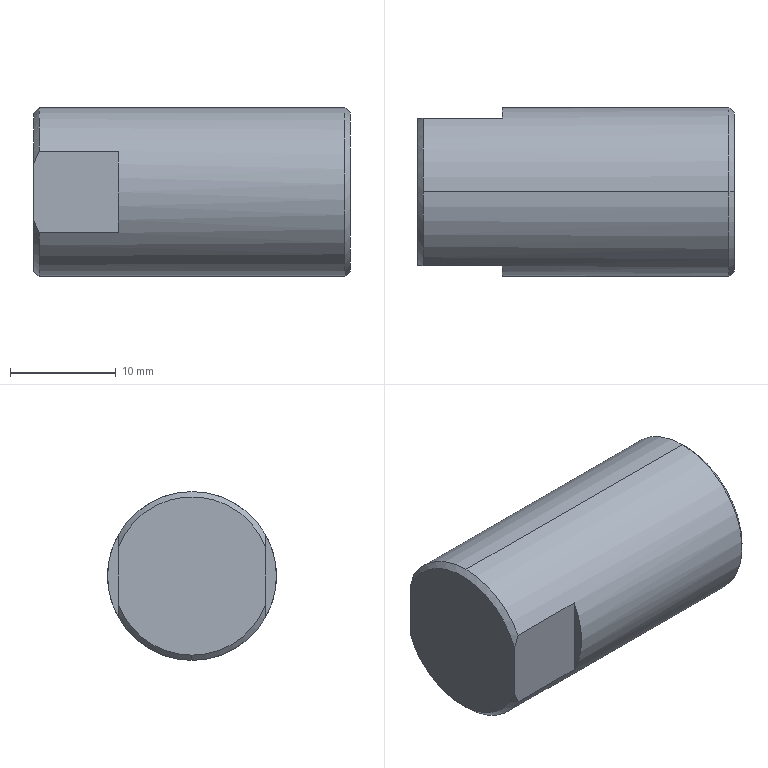Part | STEP file | PN_0024 Shaft_Default | 1 solid | 17 faces | box 30 x 16 x 16 mm | volume 5731 mm3 | cone 7 | plane 6 | cylinder 4 | commonest cylinder face diameters 5 x2 16 x2
STEP:
#1=CARTESIAN_POINT('',(0.,0.,0.));
#2=DIRECTION('',(0.,0.,1.));
#3=DIRECTION('',(1.,0.,0.));
#4=AXIS2_PLACEMENT_3D('',#1,#2,#3);
#5=CARTESIAN_POINT('',(20.,0.,-2.5));
#6=VERTEX_POINT('',#5);
#7=CARTESIAN_POINT('',(30.,0.,-2.5));
#8=VERTEX_POINT('',#7);
#9=CARTESIAN_POINT('',(30.,0.,-2.5));
#10=DIRECTION('',(1.,0.,0.));
#11=VECTOR('',#10,1.);
#12=LINE('',#9,#11);
#13=CARTESIAN_POINT('',(30.,0.,0.));
#14=DIRECTION('',(1.,0.,0.));
#15=DIRECTION('',(0.,0.,-1.));
#16=AXIS2_PLACEMENT_3D('',#13,#14,#15);
#17=CYLINDRICAL_SURFACE('',#16,2.5);
#18=CARTESIAN_POINT('',(6.283,0.));
#19=DIRECTION('',(0.,1.));
#20=VECTOR('',#19,1.);
#21=LINE('',#18,#20);
#22=(GEOMETRIC_REPRESENTATION_CONTEXT(2)PARAMETRIC_REPRESENTATION_CONTEXT()REPRESENTATION_CONTEXT('',''));
#23=DEFINITIONAL_REPRESENTATION('',(#21),#22);
#24=PCURVE('',#17,#23);
#25=CARTESIAN_POINT('',(30.,0.,0.));
#26=DIRECTION('',(1.,0.,0.));
#27=DIRECTION('',(0.,0.,-1.));
#28=AXIS2_PLACEMENT_3D('',#25,#26,#27);
#29=CYLINDRICAL_SURFACE('',#28,2.5);
#30=CARTESIAN_POINT('',(0.,0.));
#31=DIRECTION('',(0.,1.));
#32=VECTOR('',#31,1.);
#33=LINE('',#30,#32);
#34=(GEOMETRIC_REPRESENTATION_CONTEXT(2)PARAMETRIC_REPRESENTATION_CONTEXT()REPRESENTATION_CONTEXT('',''));
#35=DEFINITIONAL_REPRESENTATION('',(#33),#34);
#36=PCURVE('',#29,#35);
#37=SURFACE_CURVE('',#12,(#24,#36),.PCURVE_S1.);
#38=EDGE_CURVE('',#6,#8,#37,.T.);
#39=ORIENTED_EDGE('',*,*,#38,.T.);
#40=CARTESIAN_POINT('',(30.,0.,2.5));
#41=VERTEX_POINT('',#40);
#42=CARTESIAN_POINT('',(30.,0.,0.));
#43=DIRECTION('',(1.,0.,0.));
#44=DIRECTION('',(0.,0.,-1.));
#45=AXIS2_PLACEMENT_3D('',#42,#43,#44);
#46=CIRCLE('',#45,2.5);
#47=CARTESIAN_POINT('',(0.,0.));
#48=DIRECTION('',(1.,0.));
#49=VECTOR('',#48,1.);
#50=LINE('',#47,#49);
#51=(GEOMETRIC_REPRESENTATION_CONTEXT(2)PARAMETRIC_REPRESENTATION_CONTEXT()REPRESENTATION_CONTEXT('',''));
#52=DEFINITIONAL_REPRESENTATION('',(#50),#51);
#53=PCURVE('',#17,#52);
#54=CARTESIAN_POINT('',(30.,0.,0.));
#55=DIRECTION('',(1.,0.,0.));
#56=DIRECTION('',(0.,0.,-1.));
#57=AXIS2_PLACEMENT_3D('',#54,#55,#56);
#58=PLANE('',#57);
#59=CARTESIAN_POINT('',(0.,0.));
#60=DIRECTION('',(1.,0.));
#61=AXIS2_PLACEMENT_2D('',#59,#60);
#62=CIRCLE('',#61,2.5);
#63=(GEOMETRIC_REPRESENTATION_CONTEXT(2)PARAMETRIC_REPRESENTATION_CONTEXT()REPRESENTATION_CONTEXT('',''));
#64=DEFINITIONAL_REPRESENTATION('',(#62),#63);
#65=PCURVE('',#58,#64);
#66=SURFACE_CURVE('',#46,(#53,#65),.PCURVE_S1.);
#67=EDGE_CURVE('',#41,#8,#66,.T.);
#68=ORIENTED_EDGE('',*,*,#67,.F.);
#69=CARTESIAN_POINT('',(20.,0.,2.5));
#70=VERTEX_POINT('',#69);
#71=CARTESIAN_POINT('',(30.,0.,2.5));
#72=DIRECTION('',(1.,0.,0.));
#73=VECTOR('',#72,1.);
#74=LINE('',#71,#73);
#75=CARTESIAN_POINT('',(3.142,0.));
#76=DIRECTION('',(0.,1.));
#77=VECTOR('',#76,1.);
#78=LINE('',#75,#77);
#79=(GEOMETRIC_REPRESENTATION_CONTEXT(2)PARAMETRIC_REPRESENTATION_CONTEXT()REPRESENTATION_CONTEXT('',''));
#80=DEFINITIONAL_REPRESENTATION('',(#78),#79);
#81=PCURVE('',#17,#80);
#82=CARTESIAN_POINT('',(3.142,0.));
#83=DIRECTION('',(0.,1.));
#84=VECTOR('',#83,1.);
#85=LINE('',#82,#84);
#86=(GEOMETRIC_REPRESENTATION_CONTEXT(2)PARAMETRIC_REPRESENTATION_CONTEXT()REPRESENTATION_CONTEXT('',''));
#87=DEFINITIONAL_REPRESENTATION('',(#85),#86);
#88=PCURVE('',#29,#87);
#89=SURFACE_CURVE('',#74,(#81,#88),.PCURVE_S1.);
#90=EDGE_CURVE('',#70,#41,#89,.T.);
#91=ORIENTED_EDGE('',*,*,#90,.F.);
#92=CARTESIAN_POINT('',(20.,0.,0.));
#93=DIRECTION('',(1.,0.,0.));
#94=DIRECTION('',(0.,0.,-1.));
#95=AXIS2_PLACEMENT_3D('',#92,#93,#94);
#96=CIRCLE('',#95,2.5);
#97=CARTESIAN_POINT('',(0.,-10.));
#98=DIRECTION('',(1.,0.));
#99=VECTOR('',#98,1.);
#100=LINE('',#97,#99);
#101=(GEOMETRIC_REPRESENTATION_CONTEXT(2)PARAMETRIC_REPRESENTATION_CONTEXT()REPRESENTATION_CONTEXT('',''));
#102=DEFINITIONAL_REPRESENTATION('',(#100),#101);
#103=PCURVE('',#17,#102);
#104=CARTESIAN_POINT('',(20.,0.,0.));
#105=DIRECTION('',(1.,0.,0.));
#106=DIRECTION('',(0.,0.,-1.));
#107=AXIS2_PLACEMENT_3D('',#104,#105,#106);
#108=CONICAL_SURFACE('',#107,2.5,1.03);
#109=CARTESIAN_POINT('',(0.,0.));
#110=DIRECTION('',(1.,0.));
#111=VECTOR('',#110,1.);
#112=LINE('',#109,#111);
#113=(GEOMETRIC_REPRESENTATION_CONTEXT(2)PARAMETRIC_REPRESENTATION_CONTEXT()REPRESENTATION_CONTEXT('',''));
#114=DEFINITIONAL_REPRESENTATION('',(#112),#113);
#115=PCURVE('',#108,#114);
#116=SURFACE_CURVE('',#96,(#103,#115),.PCURVE_S1.);
#117=EDGE_CURVE('',#70,#6,#116,.T.);
#118=ORIENTED_EDGE('',*,*,#117,.T.);
#119=EDGE_LOOP('',(#39,#68,#91,#118));
#120=FACE_BOUND('',#119,.F.);
#121=ADVANCED_FACE('',(#120),#17,.F.);
#122=ORIENTED_EDGE('',*,*,#117,.F.);
#123=CARTESIAN_POINT('',(18.498,0.,0.));
#124=VERTEX_POINT('',#123);
#125=CARTESIAN_POINT('',(20.,0.,2.5));
#126=DIRECTION('',(0.515,0.,0.8572));
#127=VECTOR('',#126,1.);
#128=LINE('',#125,#127);
#129=CARTESIAN_POINT('',(3.142,0.));
#130=DIRECTION('',(0.,1.));
#131=VECTOR('',#130,1.);
#132=LINE('',#129,#131);
#133=(GEOMETRIC_REPRESENTATION_CONTEXT(2)PARAMETRIC_REPRESENTATION_CONTEXT()REPRESENTATION_CONTEXT('',''));
#134=DEFINITIONAL_REPRESENTATION('',(#132),#133);
#135=PCURVE('',#108,#134);
#136=CARTESIAN_POINT('',(20.,0.,0.));
#137=DIRECTION('',(1.,0.,0.));
#138=DIRECTION('',(0.,0.,-1.));
#139=AXIS2_PLACEMENT_3D('',#136,#137,#138);
#140=CONICAL_SURFACE('',#139,2.5,1.03);
#141=CARTESIAN_POINT('',(3.142,0.));
#142=DIRECTION('',(0.,1.));
#143=VECTOR('',#142,1.);
#144=LINE('',#141,#143);
#145=(GEOMETRIC_REPRESENTATION_CONTEXT(2)PARAMETRIC_REPRESENTATION_CONTEXT()REPRESENTATION_CONTEXT('',''));
#146=DEFINITIONAL_REPRESENTATION('',(#144),#145);
#147=PCURVE('',#140,#146);
#148=SURFACE_CURVE('',#128,(#135,#147),.PCURVE_S1.);
#149=EDGE_CURVE('',#124,#70,#148,.T.);
#150=ORIENTED_EDGE('',*,*,#149,.F.);
#151=CARTESIAN_POINT('',(20.,0.,-2.5));
#152=DIRECTION('',(0.515,0.,-0.8572));
#153=VECTOR('',#152,1.);
#154=LINE('',#151,#153);
#155=CARTESIAN_POINT('',(6.283,-1.502));
#156=CARTESIAN_POINT('',(6.283,-1.479));
#157=CARTESIAN_POINT('',(6.283,-1.434));
#158=CARTESIAN_POINT('',(6.283,-1.366));
#159=CARTESIAN_POINT('',(6.283,-1.297));
#160=CARTESIAN_POINT('',(6.283,-1.229));
#161=CARTESIAN_POINT('',(6.283,-1.161));
#162=CARTESIAN_POINT('',(6.283,-1.092));
#163=CARTESIAN_POINT('',(6.283,-1.024));
#164=CARTESIAN_POINT('',(6.283,-0.9559));
#165=CARTESIAN_POINT('',(6.283,-0.8876));
#166=CARTESIAN_POINT('',(6.283,-0.8194));
#167=CARTESIAN_POINT('',(6.283,-0.7511));
#168=CARTESIAN_POINT('',(6.283,-0.6828));
#169=CARTESIAN_POINT('',(6.283,-0.6145));
#170=CARTESIAN_POINT('',(6.283,-0.5462));
#171=CARTESIAN_POINT('',(6.283,-0.478));
#172=CARTESIAN_POINT('',(6.283,-0.4097));
#173=CARTESIAN_POINT('',(6.283,-0.3414));
#174=CARTESIAN_POINT('',(6.283,-0.2731));
#175=CARTESIAN_POINT('',(6.283,-0.2048));
#176=CARTESIAN_POINT('',(6.283,-0.1366));
#177=CARTESIAN_POINT('',(6.283,-0.06828));
#178=CARTESIAN_POINT('',(6.283,-0.02276));
#179=CARTESIAN_POINT('',(6.283,0.));
#180=B_SPLINE_CURVE_WITH_KNOTS('',3,(#155,#156,#157,#158,#159,#160,#161,#162,#163,#164,#165,#166,#167,#168,#169,#170,#171,#172,#173,#174,#175,#176,#177,#178,#179),.UNSPECIFIED.,.F.,.F.,(4,1,1,1,1,1,1,1,1,1,1,1,1,1,1,1,1,1,1,1,1,1,4),(-2.917,-2.784,-2.651,-2.519,-2.386,-2.254,-2.121,-1.989,-1.856,-1.723,-1.591,-1.458,-1.326,-1.193,-1.061,-0.928,-0.7954,-0.6629,-0.5303,-0.3977,-0.2651,-0.1326,0.),.UNSPECIFIED.);
#181=(GEOMETRIC_REPRESENTATION_CONTEXT(2)PARAMETRIC_REPRESENTATION_CONTEXT()REPRESENTATION_CONTEXT('',''));
#182=DEFINITIONAL_REPRESENTATION('',(#180),#181);
#183=PCURVE('',#108,#182);
#184=CARTESIAN_POINT('',(0.,0.));
#185=DIRECTION('',(0.,1.));
#186=VECTOR('',#185,1.);
#187=LINE('',#184,#186);
#188=(GEOMETRIC_REPRESENTATION_CONTEXT(2)PARAMETRIC_REPRESENTATION_CONTEXT()REPRESENTATION_CONTEXT('',''));
#189=DEFINITIONAL_REPRESENTATION('',(#187),#188);
#190=PCURVE('',#140,#189);
#191=SURFACE_CURVE('',#154,(#183,#190),.PCURVE_S1.);
#192=EDGE_CURVE('',#124,#6,#191,.T.);
#193=ORIENTED_EDGE('',*,*,#192,.T.);
#194=EDGE_LOOP('',(#122,#150,#193));
#195=FACE_BOUND('',#194,.F.);
#196=ADVANCED_FACE('',(#195),#108,.F.);
#197=CARTESIAN_POINT('',(0.,0.,-7.5));
#198=VERTEX_POINT('',#197);
#199=CARTESIAN_POINT('',(0.,-7.,-2.693));
#200=VERTEX_POINT('',#199);
#201=CARTESIAN_POINT('',(0.,0.,0.));
#202=DIRECTION('',(-1.,0.,0.));
#203=DIRECTION('',(0.,0.,-1.));
#204=AXIS2_PLACEMENT_3D('',#201,#202,#203);
#205=CIRCLE('',#204,7.5);
#206=CARTESIAN_POINT('',(0.5,0.,0.));
#207=DIRECTION('',(1.,0.,0.));
#208=DIRECTION('',(0.,0.,-1.));
#209=AXIS2_PLACEMENT_3D('',#206,#207,#208);
#210=CONICAL_SURFACE('',#209,8.,0.7854);
#211=CARTESIAN_POINT('',(6.283,-0.5));
#212=DIRECTION('',(-1.,0.));
#213=VECTOR('',#212,1.);
#214=LINE('',#211,#213);
#215=(GEOMETRIC_REPRESENTATION_CONTEXT(2)PARAMETRIC_REPRESENTATION_CONTEXT()REPRESENTATION_CONTEXT('',''));
#216=DEFINITIONAL_REPRESENTATION('',(#214),#215);
#217=PCURVE('',#210,#216);
#218=CARTESIAN_POINT('',(0.,0.,0.));
#219=DIRECTION('',(1.,0.,0.));
#220=DIRECTION('',(0.,0.,-1.));
#221=AXIS2_PLACEMENT_3D('',#218,#219,#220);
#222=PLANE('',#221);
#223=CARTESIAN_POINT('',(7.5,0.));
#224=CARTESIAN_POINT('',(7.5,-12.99));
#225=CARTESIAN_POINT('',(-3.75,-6.495));
#226=CARTESIAN_POINT('',(-15.,0.));
#227=CARTESIAN_POINT('',(-3.75,6.495));
#228=CARTESIAN_POINT('',(7.5,12.99));
#229=CARTESIAN_POINT('',(7.5,0.));
#230=(BOUNDED_CURVE()B_SPLINE_CURVE(2,(#223,#224,#225,#226,#227,#228,#229),.UNSPECIFIED.,.T.,.F.)B_SPLINE_CURVE_WITH_KNOTS((1,2,2,2,2,1),(-2.094,0.,2.094,4.189,6.283,8.378),.UNSPECIFIED.)CURVE()GEOMETRIC_REPRESENTATION_ITEM()RATIONAL_B_SPLINE_CURVE((1.,0.5,1.,0.5,1.,0.5,1.))REPRESENTATION_ITEM(''));
#231=(GEOMETRIC_REPRESENTATION_CONTEXT(2)PARAMETRIC_REPRESENTATION_CONTEXT()REPRESENTATION_CONTEXT('',''));
#232=DEFINITIONAL_REPRESENTATION('',(#230),#231);
#233=PCURVE('',#222,#232);
#234=SURFACE_CURVE('',#205,(#217,#233),.PCURVE_S1.);
#235=EDGE_CURVE('',#198,#200,#234,.T.);
#236=ORIENTED_EDGE('',*,*,#235,.F.);
#237=CARTESIAN_POINT('',(0.5,0.,-8.));
#238=VERTEX_POINT('',#237);
#239=CARTESIAN_POINT('',(0.5,0.,-8.));
#240=DIRECTION('',(0.7071,0.,-0.7071));
#241=VECTOR('',#240,1.);
#242=LINE('',#239,#241);
#243=CARTESIAN_POINT('',(6.283,0.));
#244=DIRECTION('',(0.,1.));
#245=VECTOR('',#244,1.);
#246=LINE('',#243,#245);
#247=(GEOMETRIC_REPRESENTATION_CONTEXT(2)PARAMETRIC_REPRESENTATION_CONTEXT()REPRESENTATION_CONTEXT('',''));
#248=DEFINITIONAL_REPRESENTATION('',(#246),#247);
#249=PCURVE('',#210,#248);
#250=CARTESIAN_POINT('',(0.5,0.,0.));
#251=DIRECTION('',(1.,0.,0.));
#252=DIRECTION('',(0.,0.,-1.));
#253=AXIS2_PLACEMENT_3D('',#250,#251,#252);
#254=CONICAL_SURFACE('',#253,8.,0.7854);
#255=CARTESIAN_POINT('',(0.,0.));
#256=DIRECTION('',(0.,1.));
#257=VECTOR('',#256,1.);
#258=LINE('',#255,#257);
#259=(GEOMETRIC_REPRESENTATION_CONTEXT(2)PARAMETRIC_REPRESENTATION_CONTEXT()REPRESENTATION_CONTEXT('',''));
#260=DEFINITIONAL_REPRESENTATION('',(#258),#259);
#261=PCURVE('',#254,#260);
#262=SURFACE_CURVE('',#242,(#249,#261),.PCURVE_S1.);
#263=EDGE_CURVE('',#198,#238,#262,.T.);
#264=ORIENTED_EDGE('',*,*,#263,.T.);
#265=CARTESIAN_POINT('',(0.5,-7.,-3.873));
#266=VERTEX_POINT('',#265);
#267=CARTESIAN_POINT('',(0.5,0.,0.));
#268=DIRECTION('',(1.,0.,0.));
#269=DIRECTION('',(0.,0.,-1.));
#270=AXIS2_PLACEMENT_3D('',#267,#268,#269);
#271=CIRCLE('',#270,8.);
#272=CARTESIAN_POINT('',(0.,0.));
#273=DIRECTION('',(1.,0.));
#274=VECTOR('',#273,1.);
#275=LINE('',#272,#274);
#276=(GEOMETRIC_REPRESENTATION_CONTEXT(2)PARAMETRIC_REPRESENTATION_CONTEXT()REPRESENTATION_CONTEXT('',''));
#277=DEFINITIONAL_REPRESENTATION('',(#275),#276);
#278=PCURVE('',#210,#277);
#279=CARTESIAN_POINT('',(30.,0.,0.));
#280=DIRECTION('',(-1.,0.,0.));
#281=DIRECTION('',(0.,0.,1.));
#282=AXIS2_PLACEMENT_3D('',#279,#280,#281);
#283=CYLINDRICAL_SURFACE('',#282,8.);
#284=CARTESIAN_POINT('',(9.425,29.5));
#285=DIRECTION('',(-1.,0.));
#286=VECTOR('',#285,1.);
#287=LINE('',#284,#286);
#288=(GEOMETRIC_REPRESENTATION_CONTEXT(2)PARAMETRIC_REPRESENTATION_CONTEXT()REPRESENTATION_CONTEXT('',''));
#289=DEFINITIONAL_REPRESENTATION('',(#287),#288);
#290=PCURVE('',#283,#289);
#291=SURFACE_CURVE('',#271,(#278,#290),.PCURVE_S1.);
#292=EDGE_CURVE('',#266,#238,#291,.T.);
#293=ORIENTED_EDGE('',*,*,#292,.F.);
#294=CARTESIAN_POINT('',(0.,-7.,-2.693));
#295=CARTESIAN_POINT('',(0.1454,-7.,-3.098));
#296=CARTESIAN_POINT('',(0.3148,-7.,-3.491));
#297=CARTESIAN_POINT('',(0.5,-7.,-3.873));
#298=B_SPLINE_CURVE_WITH_KNOTS('',3,(#294,#295,#296,#297),.UNSPECIFIED.,.F.,.F.,(4,4),(0.02242,0.02371),.PIECEWISE_BEZIER_KNOTS.);
#299=CARTESIAN_POINT('',(5.08,-0.5));
#300=CARTESIAN_POINT('',(5.082,-0.4934));
#301=CARTESIAN_POINT('',(5.086,-0.4801));
#302=CARTESIAN_POINT('',(5.093,-0.4598));
#303=CARTESIAN_POINT('',(5.1,-0.4392));
#304=CARTESIAN_POINT('',(5.107,-0.4184));
#305=CARTESIAN_POINT('',(5.113,-0.3973));
#306=CARTESIAN_POINT('',(5.12,-0.3759));
#307=CARTESIAN_POINT('',(5.126,-0.3542));
#308=CARTESIAN_POINT('',(5.133,-0.3323));
#309=CARTESIAN_POINT('',(5.139,-0.3101));
#310=CARTESIAN_POINT('',(5.146,-0.2876));
#311=CARTESIAN_POINT('',(5.152,-0.2649));
#312=CARTESIAN_POINT('',(5.158,-0.242));
#313=CARTESIAN_POINT('',(5.164,-0.2188));
#314=CARTESIAN_POINT('',(5.17,-0.1954));
#315=CARTESIAN_POINT('',(5.177,-0.1717));
#316=CARTESIAN_POINT('',(5.183,-0.1478));
#317=CARTESIAN_POINT('',(5.189,-0.1237));
#318=CARTESIAN_POINT('',(5.195,-0.09942));
#319=CARTESIAN_POINT('',(5.2,-0.07488));
#320=CARTESIAN_POINT('',(5.206,-0.05013));
#321=CARTESIAN_POINT('',(5.212,-0.02518));
#322=CARTESIAN_POINT('',(5.216,-0.008416));
#323=CARTESIAN_POINT('',(5.218,0.));
#324=B_SPLINE_CURVE_WITH_KNOTS('',3,(#299,#300,#301,#302,#303,#304,#305,#306,#307,#308,#309,#310,#311,#312,#313,#314,#315,#316,#317,#318,#319,#320,#321,#322,#323),.UNSPECIFIED.,.F.,.F.,(4,1,1,1,1,1,1,1,1,1,1,1,1,1,1,1,1,1,1,1,1,1,4),(0.02242,0.02248,0.02254,0.0226,0.02266,0.02272,0.02277,0.02283,0.02289,0.02295,0.02301,0.02307,0.02312,0.02318,0.02324,0.0233,0.02336,0.02342,0.02347,0.02353,0.02359,0.02365,0.02371),.QUASI_UNIFORM_KNOTS.);
#325=(GEOMETRIC_REPRESENTATION_CONTEXT(2)PARAMETRIC_REPRESENTATION_CONTEXT()REPRESENTATION_CONTEXT('',''));
#326=DEFINITIONAL_REPRESENTATION('',(#324),#325);
#327=PCURVE('',#210,#326);
#328=CARTESIAN_POINT('',(0.,-7.,-18.));
#329=DIRECTION('',(0.,1.,0.));
#330=DIRECTION('',(0.,0.,1.));
#331=AXIS2_PLACEMENT_3D('',#328,#329,#330);
#332=PLANE('',#331);
#333=CARTESIAN_POINT('',(15.307,0.));
#334=CARTESIAN_POINT('',(14.902,0.1454));
#335=CARTESIAN_POINT('',(14.509,0.3148));
#336=CARTESIAN_POINT('',(14.127,0.5));
#337=B_SPLINE_CURVE_WITH_KNOTS('',3,(#333,#334,#335,#336),.UNSPECIFIED.,.F.,.F.,(4,4),(0.02242,0.02371),.PIECEWISE_BEZIER_KNOTS.);
#338=(GEOMETRIC_REPRESENTATION_CONTEXT(2)PARAMETRIC_REPRESENTATION_CONTEXT()REPRESENTATION_CONTEXT('',''));
#339=DEFINITIONAL_REPRESENTATION('',(#337),#338);
#340=PCURVE('',#332,#339);
#341=SURFACE_CURVE('',#298,(#327,#340),.PCURVE_S1.);
#342=EDGE_CURVE('',#200,#266,#341,.T.);
#343=ORIENTED_EDGE('',*,*,#342,.F.);
#344=EDGE_LOOP('',(#236,#264,#293,#343));
#345=FACE_BOUND('',#344,.T.);
#346=ADVANCED_FACE('',(#345),#210,.T.);
#347=CARTESIAN_POINT('',(30.,0.,-7.5));
#348=VERTEX_POINT('',#347);
#349=CARTESIAN_POINT('',(30.,0.,7.5));
#350=VERTEX_POINT('',#349);
#351=CARTESIAN_POINT('',(30.,0.,0.));
#352=DIRECTION('',(1.,0.,0.));
#353=DIRECTION('',(0.,0.,-1.));
#354=AXIS2_PLACEMENT_3D('',#351,#352,#353);
#355=CIRCLE('',#354,7.5);
#356=CARTESIAN_POINT('',(30.,0.,0.));
#357=DIRECTION('',(-1.,0.,0.));
#358=DIRECTION('',(0.,0.,1.));
#359=AXIS2_PLACEMENT_3D('',#356,#357,#358);
#360=CONICAL_SURFACE('',#359,7.5,0.7854);
#361=CARTESIAN_POINT('',(3.142,0.));
#362=DIRECTION('',(-1.,0.));
#363=VECTOR('',#362,1.);
#364=LINE('',#361,#363);
#365=(GEOMETRIC_REPRESENTATION_CONTEXT(2)PARAMETRIC_REPRESENTATION_CONTEXT()REPRESENTATION_CONTEXT('',''));
#366=DEFINITIONAL_REPRESENTATION('',(#364),#365);
#367=PCURVE('',#360,#366);
#368=CARTESIAN_POINT('',(0.,0.));
#369=DIRECTION('',(1.,0.));
#370=AXIS2_PLACEMENT_2D('',#368,#369);
#371=CIRCLE('',#370,7.5);
#372=(GEOMETRIC_REPRESENTATION_CONTEXT(2)PARAMETRIC_REPRESENTATION_CONTEXT()REPRESENTATION_CONTEXT('',''));
#373=DEFINITIONAL_REPRESENTATION('',(#371),#372);
#374=PCURVE('',#58,#373);
#375=SURFACE_CURVE('',#355,(#367,#374),.PCURVE_S1.);
#376=EDGE_CURVE('',#348,#350,#375,.T.);
#377=ORIENTED_EDGE('',*,*,#376,.F.);
#378=CARTESIAN_POINT('',(29.5,0.,-8.));
#379=VERTEX_POINT('',#378);
#380=CARTESIAN_POINT('',(30.,0.,-7.5));
#381=DIRECTION('',(-0.7071,0.,-0.7071));
#382=VECTOR('',#381,1.);
#383=LINE('',#380,#382);
#384=CARTESIAN_POINT('',(3.142,0.));
#385=DIRECTION('',(0.,1.));
#386=VECTOR('',#385,1.);
#387=LINE('',#384,#386);
#388=(GEOMETRIC_REPRESENTATION_CONTEXT(2)PARAMETRIC_REPRESENTATION_CONTEXT()REPRESENTATION_CONTEXT('',''));
#389=DEFINITIONAL_REPRESENTATION('',(#387),#388);
#390=PCURVE('',#360,#389);
#391=CARTESIAN_POINT('',(30.,0.,0.));
#392=DIRECTION('',(-1.,0.,0.));
#393=DIRECTION('',(0.,0.,1.));
#394=AXIS2_PLACEMENT_3D('',#391,#392,#393);
#395=CONICAL_SURFACE('',#394,7.5,0.7854);
#396=CARTESIAN_POINT('',(3.142,0.));
#397=DIRECTION('',(0.,1.));
#398=VECTOR('',#397,1.);
#399=LINE('',#396,#398);
#400=(GEOMETRIC_REPRESENTATION_CONTEXT(2)PARAMETRIC_REPRESENTATION_CONTEXT()REPRESENTATION_CONTEXT('',''));
#401=DEFINITIONAL_REPRESENTATION('',(#399),#400);
#402=PCURVE('',#395,#401);
#403=SURFACE_CURVE('',#383,(#390,#402),.PCURVE_S1.);
#404=EDGE_CURVE('',#348,#379,#403,.T.);
#405=ORIENTED_EDGE('',*,*,#404,.T.);
#406=CARTESIAN_POINT('',(29.5,0.,8.));
#407=VERTEX_POINT('',#406);
#408=CARTESIAN_POINT('',(29.5,0.,0.));
#409=DIRECTION('',(-1.,0.,0.));
#410=DIRECTION('',(0.,0.,-1.));
#411=AXIS2_PLACEMENT_3D('',#408,#409,#410);
#412=CIRCLE('',#411,8.);
#413=CARTESIAN_POINT('',(-3.142,0.5));
#414=DIRECTION('',(1.,0.));
#415=VECTOR('',#414,1.);
#416=LINE('',#413,#415);
#417=(GEOMETRIC_REPRESENTATION_CONTEXT(2)PARAMETRIC_REPRESENTATION_CONTEXT()REPRESENTATION_CONTEXT('',''));
#418=DEFINITIONAL_REPRESENTATION('',(#416),#417);
#419=PCURVE('',#360,#418);
#420=CARTESIAN_POINT('',(30.,0.,0.));
#421=DIRECTION('',(-1.,0.,0.));
#422=DIRECTION('',(0.,0.,1.));
#423=AXIS2_PLACEMENT_3D('',#420,#421,#422);
#424=CYLINDRICAL_SURFACE('',#423,8.);
#425=CARTESIAN_POINT('',(-3.142,0.5));
#426=DIRECTION('',(1.,0.));
#427=VECTOR('',#426,1.);
#428=LINE('',#425,#427);
#429=(GEOMETRIC_REPRESENTATION_CONTEXT(2)PARAMETRIC_REPRESENTATION_CONTEXT()REPRESENTATION_CONTEXT('',''));
#430=DEFINITIONAL_REPRESENTATION('',(#428),#429);
#431=PCURVE('',#424,#430);
#432=SURFACE_CURVE('',#412,(#419,#431),.PCURVE_S1.);
#433=EDGE_CURVE('',#407,#379,#432,.T.);
#434=ORIENTED_EDGE('',*,*,#433,.F.);
#435=CARTESIAN_POINT('',(30.,0.,7.5));
#436=DIRECTION('',(-0.7071,0.,0.7071));
#437=VECTOR('',#436,1.);
#438=LINE('',#435,#437);
#439=CARTESIAN_POINT('',(0.,0.));
#440=DIRECTION('',(0.,1.));
#441=VECTOR('',#440,1.);
#442=LINE('',#439,#441);
#443=(GEOMETRIC_REPRESENTATION_CONTEXT(2)PARAMETRIC_REPRESENTATION_CONTEXT()REPRESENTATION_CONTEXT('',''));
#444=DEFINITIONAL_REPRESENTATION('',(#442),#443);
#445=PCURVE('',#360,#444);
#446=CARTESIAN_POINT('',(6.283,0.));
#447=DIRECTION('',(0.,1.));
#448=VECTOR('',#447,1.);
#449=LINE('',#446,#448);
#450=(GEOMETRIC_REPRESENTATION_CONTEXT(2)PARAMETRIC_REPRESENTATION_CONTEXT()REPRESENTATION_CONTEXT('',''));
#451=DEFINITIONAL_REPRESENTATION('',(#449),#450);
#452=PCURVE('',#395,#451);
#453=SURFACE_CURVE('',#438,(#445,#452),.PCURVE_S1.);
#454=EDGE_CURVE('',#350,#407,#453,.T.);
#455=ORIENTED_EDGE('',*,*,#454,.F.);
#456=EDGE_LOOP('',(#377,#405,#434,#455));
#457=FACE_BOUND('',#456,.T.);
#458=ADVANCED_FACE('',(#457),#360,.T.);
#459=ORIENTED_EDGE('',*,*,#433,.T.);
#460=CARTESIAN_POINT('',(30.,0.,-8.));
#461=DIRECTION('',(-1.,0.,0.));
#462=VECTOR('',#461,1.);
#463=LINE('',#460,#462);
#464=CARTESIAN_POINT('',(3.142,0.));
#465=DIRECTION('',(0.,1.));
#466=VECTOR('',#465,1.);
#467=LINE('',#464,#466);
#468=(GEOMETRIC_REPRESENTATION_CONTEXT(2)PARAMETRIC_REPRESENTATION_CONTEXT()REPRESENTATION_CONTEXT('',''));
#469=DEFINITIONAL_REPRESENTATION('',(#467),#468);
#470=PCURVE('',#424,#469);
#471=CARTESIAN_POINT('',(3.142,0.));
#472=DIRECTION('',(0.,1.));
#473=VECTOR('',#472,1.);
#474=LINE('',#471,#473);
#475=(GEOMETRIC_REPRESENTATION_CONTEXT(2)PARAMETRIC_REPRESENTATION_CONTEXT()REPRESENTATION_CONTEXT('',''));
#476=DEFINITIONAL_REPRESENTATION('',(#474),#475);
#477=PCURVE('',#283,#476);
#478=SURFACE_CURVE('',#463,(#470,#477),.PCURVE_S1.);
#479=EDGE_CURVE('',#379,#238,#478,.T.);
#480=ORIENTED_EDGE('',*,*,#479,.T.);
#481=CARTESIAN_POINT('',(0.5,7.,-3.873));
#482=VERTEX_POINT('',#481);
#483=CARTESIAN_POINT('',(0.5,0.,0.));
#484=DIRECTION('',(1.,0.,0.));
#485=DIRECTION('',(0.,0.,-1.));
#486=AXIS2_PLACEMENT_3D('',#483,#484,#485);
#487=CIRCLE('',#486,8.);
#488=CARTESIAN_POINT('',(3.142,29.5));
#489=DIRECTION('',(-1.,0.));
#490=VECTOR('',#489,1.);
#491=LINE('',#488,#490);
#492=(GEOMETRIC_REPRESENTATION_CONTEXT(2)PARAMETRIC_REPRESENTATION_CONTEXT()REPRESENTATION_CONTEXT('',''));
#493=DEFINITIONAL_REPRESENTATION('',(#491),#492);
#494=PCURVE('',#424,#493);
#495=CARTESIAN_POINT('',(0.,0.));
#496=DIRECTION('',(1.,0.));
#497=VECTOR('',#496,1.);
#498=LINE('',#495,#497);
#499=(GEOMETRIC_REPRESENTATION_CONTEXT(2)PARAMETRIC_REPRESENTATION_CONTEXT()REPRESENTATION_CONTEXT('',''));
#500=DEFINITIONAL_REPRESENTATION('',(#498),#499);
#501=PCURVE('',#254,#500);
#502=SURFACE_CURVE('',#487,(#494,#501),.PCURVE_S1.);
#503=EDGE_CURVE('',#238,#482,#502,.T.);
#504=ORIENTED_EDGE('',*,*,#503,.T.);
#505=CARTESIAN_POINT('',(8.,7.,-3.873));
#506=VERTEX_POINT('',#505);
#507=CARTESIAN_POINT('',(30.,7.,-3.873));
#508=DIRECTION('',(1.,0.,0.));
#509=VECTOR('',#508,1.);
#510=LINE('',#507,#509);
#511=CARTESIAN_POINT('',(2.076,0.));
#512=DIRECTION('',(0.,-1.));
#513=VECTOR('',#512,1.);
#514=LINE('',#511,#513);
#515=(GEOMETRIC_REPRESENTATION_CONTEXT(2)PARAMETRIC_REPRESENTATION_CONTEXT()REPRESENTATION_CONTEXT('',''));
#516=DEFINITIONAL_REPRESENTATION('',(#514),#515);
#517=PCURVE('',#424,#516);
#518=CARTESIAN_POINT('',(0.,7.,-18.));
#519=DIRECTION('',(0.,-1.,0.));
#520=DIRECTION('',(0.,0.,-1.));
#521=AXIS2_PLACEMENT_3D('',#518,#519,#520);
#522=PLANE('',#521);
#523=CARTESIAN_POINT('',(-14.127,30.));
#524=DIRECTION('',(0.,1.));
#525=VECTOR('',#524,1.);
#526=LINE('',#523,#525);
#527=(GEOMETRIC_REPRESENTATION_CONTEXT(2)PARAMETRIC_REPRESENTATION_CONTEXT()REPRESENTATION_CONTEXT('',''));
#528=DEFINITIONAL_REPRESENTATION('',(#526),#527);
#529=PCURVE('',#522,#528);
#530=SURFACE_CURVE('',#510,(#517,#529),.PCURVE_S1.);
#531=EDGE_CURVE('',#482,#506,#530,.T.);
#532=ORIENTED_EDGE('',*,*,#531,.T.);
#533=CARTESIAN_POINT('',(8.,7.,3.873));
#534=VERTEX_POINT('',#533);
#535=CARTESIAN_POINT('',(8.,0.,0.));
#536=DIRECTION('',(1.,0.,0.));
#537=DIRECTION('',(0.,0.,-1.));
#538=AXIS2_PLACEMENT_3D('',#535,#536,#537);
#539=CIRCLE('',#538,8.);
#540=CARTESIAN_POINT('',(3.142,22.));
#541=DIRECTION('',(-1.,0.));
#542=VECTOR('',#541,1.);
#543=LINE('',#540,#542);
#544=(GEOMETRIC_REPRESENTATION_CONTEXT(2)PARAMETRIC_REPRESENTATION_CONTEXT()REPRESENTATION_CONTEXT('',''));
#545=DEFINITIONAL_REPRESENTATION('',(#543),#544);
#546=PCURVE('',#424,#545);
#547=CARTESIAN_POINT('',(8.,10.071,-18.));
#548=DIRECTION('',(1.,0.,0.));
#549=DIRECTION('',(0.,0.,-1.));
#550=AXIS2_PLACEMENT_3D('',#547,#548,#549);
#551=PLANE('',#550);
#552=CARTESIAN_POINT('',(-18.,-10.071));
#553=DIRECTION('',(1.,0.));
#554=AXIS2_PLACEMENT_2D('',#552,#553);
#555=CIRCLE('',#554,8.);
#556=(GEOMETRIC_REPRESENTATION_CONTEXT(2)PARAMETRIC_REPRESENTATION_CONTEXT()REPRESENTATION_CONTEXT('',''));
#557=DEFINITIONAL_REPRESENTATION('',(#555),#556);
#558=PCURVE('',#551,#557);
#559=SURFACE_CURVE('',#539,(#546,#558),.PCURVE_S1.);
#560=EDGE_CURVE('',#506,#534,#559,.T.);
#561=ORIENTED_EDGE('',*,*,#560,.T.);
#562=CARTESIAN_POINT('',(0.5,7.,3.873));
#563=VERTEX_POINT('',#562);
#564=CARTESIAN_POINT('',(30.,7.,3.873));
#565=DIRECTION('',(-1.,0.,0.));
#566=VECTOR('',#565,1.);
#567=LINE('',#564,#566);
#568=CARTESIAN_POINT('',(1.065,0.));
#569=DIRECTION('',(0.,1.));
#570=VECTOR('',#569,1.);
#571=LINE('',#568,#570);
#572=(GEOMETRIC_REPRESENTATION_CONTEXT(2)PARAMETRIC_REPRESENTATION_CONTEXT()REPRESENTATION_CONTEXT('',''));
#573=DEFINITIONAL_REPRESENTATION('',(#571),#572);
#574=PCURVE('',#424,#573);
#575=CARTESIAN_POINT('',(-21.873,30.));
#576=DIRECTION('',(0.,-1.));
#577=VECTOR('',#576,1.);
#578=LINE('',#575,#577);
#579=(GEOMETRIC_REPRESENTATION_CONTEXT(2)PARAMETRIC_REPRESENTATION_CONTEXT()REPRESENTATION_CONTEXT('',''));
#580=DEFINITIONAL_REPRESENTATION('',(#578),#579);
#581=PCURVE('',#522,#580);
#582=SURFACE_CURVE('',#567,(#574,#581),.PCURVE_S1.);
#583=EDGE_CURVE('',#534,#563,#582,.T.);
#584=ORIENTED_EDGE('',*,*,#583,.T.);
#585=CARTESIAN_POINT('',(0.5,0.,8.));
#586=VERTEX_POINT('',#585);
#587=CARTESIAN_POINT('',(0.5,0.,0.));
#588=DIRECTION('',(1.,0.,0.));
#589=DIRECTION('',(0.,0.,-1.));
#590=AXIS2_PLACEMENT_3D('',#587,#588,#589);
#591=CIRCLE('',#590,8.);
#592=CARTESIAN_POINT('',(3.142,29.5));
#593=DIRECTION('',(-1.,0.));
#594=VECTOR('',#593,1.);
#595=LINE('',#592,#594);
#596=(GEOMETRIC_REPRESENTATION_CONTEXT(2)PARAMETRIC_REPRESENTATION_CONTEXT()REPRESENTATION_CONTEXT('',''));
#597=DEFINITIONAL_REPRESENTATION('',(#595),#596);
#598=PCURVE('',#424,#597);
#599=CARTESIAN_POINT('',(0.5,0.,0.));
#600=DIRECTION('',(1.,0.,0.));
#601=DIRECTION('',(0.,0.,-1.));
#602=AXIS2_PLACEMENT_3D('',#599,#600,#601);
#603=CONICAL_SURFACE('',#602,8.,0.7854);
#604=CARTESIAN_POINT('',(0.,0.));
#605=DIRECTION('',(1.,0.));
#606=VECTOR('',#605,1.);
#607=LINE('',#604,#606);
#608=(GEOMETRIC_REPRESENTATION_CONTEXT(2)PARAMETRIC_REPRESENTATION_CONTEXT()REPRESENTATION_CONTEXT('',''));
#609=DEFINITIONAL_REPRESENTATION('',(#607),#608);
#610=PCURVE('',#603,#609);
#611=SURFACE_CURVE('',#591,(#598,#610),.PCURVE_S1.);
#612=EDGE_CURVE('',#563,#586,#611,.T.);
#613=ORIENTED_EDGE('',*,*,#612,.T.);
#614=CARTESIAN_POINT('',(30.,0.,8.));
#615=DIRECTION('',(-1.,0.,0.));
#616=VECTOR('',#615,1.);
#617=LINE('',#614,#616);
#618=CARTESIAN_POINT('',(0.,0.));
#619=DIRECTION('',(0.,1.));
#620=VECTOR('',#619,1.);
#621=LINE('',#618,#620);
#622=(GEOMETRIC_REPRESENTATION_CONTEXT(2)PARAMETRIC_REPRESENTATION_CONTEXT()REPRESENTATION_CONTEXT('',''));
#623=DEFINITIONAL_REPRESENTATION('',(#621),#622);
#624=PCURVE('',#424,#623);
#625=CARTESIAN_POINT('',(6.283,0.));
#626=DIRECTION('',(0.,1.));
#627=VECTOR('',#626,1.);
#628=LINE('',#625,#627);
#629=(GEOMETRIC_REPRESENTATION_CONTEXT(2)PARAMETRIC_REPRESENTATION_CONTEXT()REPRESENTATION_CONTEXT('',''));
#630=DEFINITIONAL_REPRESENTATION('',(#628),#629);
#631=PCURVE('',#283,#630);
#632=SURFACE_CURVE('',#617,(#624,#631),.PCURVE_S1.);
#633=EDGE_CURVE('',#407,#586,#632,.T.);
#634=ORIENTED_EDGE('',*,*,#633,.F.);
#635=EDGE_LOOP('',(#459,#480,#504,#532,#561,#584,#613,#634));
#636=FACE_BOUND('',#635,.T.);
#637=ADVANCED_FACE('',(#636),#424,.T.);
#638=CARTESIAN_POINT('',(0.5,-7.,3.873));
#639=VERTEX_POINT('',#638);
#640=CARTESIAN_POINT('',(0.,-7.,2.693));
#641=VERTEX_POINT('',#640);
#642=CARTESIAN_POINT('',(0.5,-7.,3.873));
#643=CARTESIAN_POINT('',(0.3138,-7.,3.488));
#644=CARTESIAN_POINT('',(0.1448,-7.,3.096));
#645=CARTESIAN_POINT('',(0.,-7.,2.693));
#646=B_SPLINE_CURVE_WITH_KNOTS('',3,(#642,#643,#644,#645),.UNSPECIFIED.,.F.,.F.,(4,4),(0.01564,0.01692),.PIECEWISE_BEZIER_KNOTS.);
#647=CARTESIAN_POINT('',(4.207,0.));
#648=CARTESIAN_POINT('',(4.209,-0.008463));
#649=CARTESIAN_POINT('',(4.213,-0.02532));
#650=CARTESIAN_POINT('',(4.219,-0.05038));
#651=CARTESIAN_POINT('',(4.224,-0.07522));
#652=CARTESIAN_POINT('',(4.23,-0.09984));
#653=CARTESIAN_POINT('',(4.236,-0.1242));
#654=CARTESIAN_POINT('',(4.242,-0.1484));
#655=CARTESIAN_POINT('',(4.248,-0.1723));
#656=CARTESIAN_POINT('',(4.254,-0.196));
#657=CARTESIAN_POINT('',(4.261,-0.2194));
#658=CARTESIAN_POINT('',(4.267,-0.2426));
#659=CARTESIAN_POINT('',(4.273,-0.2655));
#660=CARTESIAN_POINT('',(4.279,-0.2882));
#661=CARTESIAN_POINT('',(4.286,-0.3106));
#662=CARTESIAN_POINT('',(4.292,-0.3328));
#663=CARTESIAN_POINT('',(4.299,-0.3547));
#664=CARTESIAN_POINT('',(4.305,-0.3763));
#665=CARTESIAN_POINT('',(4.312,-0.3976));
#666=CARTESIAN_POINT('',(4.318,-0.4187));
#667=CARTESIAN_POINT('',(4.325,-0.4395));
#668=CARTESIAN_POINT('',(4.332,-0.46));
#669=CARTESIAN_POINT('',(4.338,-0.4802));
#670=CARTESIAN_POINT('',(4.343,-0.4934));
#671=CARTESIAN_POINT('',(4.345,-0.5));
#672=B_SPLINE_CURVE_WITH_KNOTS('',3,(#647,#648,#649,#650,#651,#652,#653,#654,#655,#656,#657,#658,#659,#660,#661,#662,#663,#664,#665,#666,#667,#668,#669,#670,#671),.UNSPECIFIED.,.F.,.F.,(4,1,1,1,1,1,1,1,1,1,1,1,1,1,1,1,1,1,1,1,1,1,4),(0.01564,0.01569,0.01575,0.01581,0.01587,0.01593,0.01599,0.01604,0.0161,0.01616,0.01622,0.01628,0.01634,0.01639,0.01645,0.01651,0.01657,0.01663,0.01669,0.01674,0.0168,0.01686,0.01692),.QUASI_UNIFORM_KNOTS.);
#673=(GEOMETRIC_REPRESENTATION_CONTEXT(2)PARAMETRIC_REPRESENTATION_CONTEXT()REPRESENTATION_CONTEXT('',''));
#674=DEFINITIONAL_REPRESENTATION('',(#672),#673);
#675=PCURVE('',#603,#674);
#676=CARTESIAN_POINT('',(21.873,0.5));
#677=CARTESIAN_POINT('',(21.488,0.3138));
#678=CARTESIAN_POINT('',(21.096,0.1448));
#679=CARTESIAN_POINT('',(20.693,0.));
#680=B_SPLINE_CURVE_WITH_KNOTS('',3,(#676,#677,#678,#679),.UNSPECIFIED.,.F.,.F.,(4,4),(0.01564,0.01692),.PIECEWISE_BEZIER_KNOTS.);
#681=(GEOMETRIC_REPRESENTATION_CONTEXT(2)PARAMETRIC_REPRESENTATION_CONTEXT()REPRESENTATION_CONTEXT('',''));
#682=DEFINITIONAL_REPRESENTATION('',(#680),#681);
#683=PCURVE('',#332,#682);
#684=SURFACE_CURVE('',#646,(#675,#683),.PCURVE_S1.);
#685=EDGE_CURVE('',#639,#641,#684,.T.);
#686=ORIENTED_EDGE('',*,*,#685,.F.);
#687=CARTESIAN_POINT('',(0.5,0.,0.));
#688=DIRECTION('',(1.,0.,0.));
#689=DIRECTION('',(0.,0.,-1.));
#690=AXIS2_PLACEMENT_3D('',#687,#688,#689);
#691=CIRCLE('',#690,8.);
#692=CARTESIAN_POINT('',(0.,0.));
#693=DIRECTION('',(1.,0.));
#694=VECTOR('',#693,1.);
#695=LINE('',#692,#694);
#696=(GEOMETRIC_REPRESENTATION_CONTEXT(2)PARAMETRIC_REPRESENTATION_CONTEXT()REPRESENTATION_CONTEXT('',''));
#697=DEFINITIONAL_REPRESENTATION('',(#695),#696);
#698=PCURVE('',#603,#697);
#699=CARTESIAN_POINT('',(9.425,29.5));
#700=DIRECTION('',(-1.,0.));
#701=VECTOR('',#700,1.);
#702=LINE('',#699,#701);
#703=(GEOMETRIC_REPRESENTATION_CONTEXT(2)PARAMETRIC_REPRESENTATION_CONTEXT()REPRESENTATION_CONTEXT('',''));
#704=DEFINITIONAL_REPRESENTATION('',(#702),#703);
#705=PCURVE('',#283,#704);
#706=SURFACE_CURVE('',#691,(#698,#705),.PCURVE_S1.);
#707=EDGE_CURVE('',#586,#639,#706,.T.);
#708=ORIENTED_EDGE('',*,*,#707,.F.);
#709=ORIENTED_EDGE('',*,*,#612,.F.);
#710=CARTESIAN_POINT('',(0.,7.,2.693));
#711=VERTEX_POINT('',#710);
#712=CARTESIAN_POINT('',(0.,7.,2.693));
#713=CARTESIAN_POINT('',(0.1454,7.,3.098));
#714=CARTESIAN_POINT('',(0.3148,7.,3.491));
#715=CARTESIAN_POINT('',(0.5,7.,3.873));
#716=B_SPLINE_CURVE_WITH_KNOTS('',3,(#712,#713,#714,#715),.UNSPECIFIED.,.F.,.F.,(4,4),(0.02242,0.02371),.PIECEWISE_BEZIER_KNOTS.);
#717=CARTESIAN_POINT('',(1.938,-0.5));
#718=CARTESIAN_POINT('',(1.94,-0.4934));
#719=CARTESIAN_POINT('',(1.945,-0.4801));
#720=CARTESIAN_POINT('',(1.952,-0.4598));
#721=CARTESIAN_POINT('',(1.958,-0.4392));
#722=CARTESIAN_POINT('',(1.965,-0.4184));
#723=CARTESIAN_POINT('',(1.972,-0.3973));
#724=CARTESIAN_POINT('',(1.978,-0.3759));
#725=CARTESIAN_POINT('',(1.985,-0.3542));
#726=CARTESIAN_POINT('',(1.991,-0.3323));
#727=CARTESIAN_POINT('',(1.998,-0.3101));
#728=CARTESIAN_POINT('',(2.004,-0.2876));
#729=CARTESIAN_POINT('',(2.01,-0.2649));
#730=CARTESIAN_POINT('',(2.017,-0.242));
#731=CARTESIAN_POINT('',(2.023,-0.2188));
#732=CARTESIAN_POINT('',(2.029,-0.1954));
#733=CARTESIAN_POINT('',(2.035,-0.1717));
#734=CARTESIAN_POINT('',(2.041,-0.1478));
#735=CARTESIAN_POINT('',(2.047,-0.1237));
#736=CARTESIAN_POINT('',(2.053,-0.09942));
#737=CARTESIAN_POINT('',(2.059,-0.07488));
#738=CARTESIAN_POINT('',(2.065,-0.05013));
#739=CARTESIAN_POINT('',(2.07,-0.02518));
#740=CARTESIAN_POINT('',(2.074,-0.008416));
#741=CARTESIAN_POINT('',(2.076,0.));
#742=B_SPLINE_CURVE_WITH_KNOTS('',3,(#717,#718,#719,#720,#721,#722,#723,#724,#725,#726,#727,#728,#729,#730,#731,#732,#733,#734,#735,#736,#737,#738,#739,#740,#741),.UNSPECIFIED.,.F.,.F.,(4,1,1,1,1,1,1,1,1,1,1,1,1,1,1,1,1,1,1,1,1,1,4),(0.02242,0.02248,0.02254,0.0226,0.02266,0.02272,0.02277,0.02283,0.02289,0.02295,0.02301,0.02307,0.02312,0.02318,0.02324,0.0233,0.02336,0.02342,0.02347,0.02353,0.02359,0.02365,0.02371),.QUASI_UNIFORM_KNOTS.);
#743=(GEOMETRIC_REPRESENTATION_CONTEXT(2)PARAMETRIC_REPRESENTATION_CONTEXT()REPRESENTATION_CONTEXT('',''));
#744=DEFINITIONAL_REPRESENTATION('',(#742),#743);
#745=PCURVE('',#603,#744);
#746=CARTESIAN_POINT('',(-20.693,0.));
#747=CARTESIAN_POINT('',(-21.098,0.1454));
#748=CARTESIAN_POINT('',(-21.491,0.3148));
#749=CARTESIAN_POINT('',(-21.873,0.5));
#750=B_SPLINE_CURVE_WITH_KNOTS('',3,(#746,#747,#748,#749),.UNSPECIFIED.,.F.,.F.,(4,4),(0.02242,0.02371),.PIECEWISE_BEZIER_KNOTS.);
#751=(GEOMETRIC_REPRESENTATION_CONTEXT(2)PARAMETRIC_REPRESENTATION_CONTEXT()REPRESENTATION_CONTEXT('',''));
#752=DEFINITIONAL_REPRESENTATION('',(#750),#751);
#753=PCURVE('',#522,#752);
#754=SURFACE_CURVE('',#716,(#745,#753),.PCURVE_S1.);
#755=EDGE_CURVE('',#711,#563,#754,.T.);
#756=ORIENTED_EDGE('',*,*,#755,.F.);
#757=CARTESIAN_POINT('',(0.,0.,0.));
#758=DIRECTION('',(-1.,0.,0.));
#759=DIRECTION('',(0.,0.,-1.));
#760=AXIS2_PLACEMENT_3D('',#757,#758,#759);
#761=CIRCLE('',#760,7.5);
#762=CARTESIAN_POINT('',(6.283,-0.5));
#763=DIRECTION('',(-1.,0.));
#764=VECTOR('',#763,1.);
#765=LINE('',#762,#764);
#766=(GEOMETRIC_REPRESENTATION_CONTEXT(2)PARAMETRIC_REPRESENTATION_CONTEXT()REPRESENTATION_CONTEXT('',''));
#767=DEFINITIONAL_REPRESENTATION('',(#765),#766);
#768=PCURVE('',#603,#767);
#769=CARTESIAN_POINT('',(7.5,0.));
#770=CARTESIAN_POINT('',(7.5,-12.99));
#771=CARTESIAN_POINT('',(-3.75,-6.495));
#772=CARTESIAN_POINT('',(-15.,0.));
#773=CARTESIAN_POINT('',(-3.75,6.495));
#774=CARTESIAN_POINT('',(7.5,12.99));
#775=CARTESIAN_POINT('',(7.5,0.));
#776=(BOUNDED_CURVE()B_SPLINE_CURVE(2,(#769,#770,#771,#772,#773,#774,#775),.UNSPECIFIED.,.T.,.F.)B_SPLINE_CURVE_WITH_KNOTS((1,2,2,2,2,1),(-2.094,0.,2.094,4.189,6.283,8.378),.UNSPECIFIED.)CURVE()GEOMETRIC_REPRESENTATION_ITEM()RATIONAL_B_SPLINE_CURVE((1.,0.5,1.,0.5,1.,0.5,1.))REPRESENTATION_ITEM(''));
#777=(GEOMETRIC_REPRESENTATION_CONTEXT(2)PARAMETRIC_REPRESENTATION_CONTEXT()REPRESENTATION_CONTEXT('',''));
#778=DEFINITIONAL_REPRESENTATION('',(#776),#777);
#779=PCURVE('',#222,#778);
#780=SURFACE_CURVE('',#761,(#768,#779),.PCURVE_S1.);
#781=EDGE_CURVE('',#641,#711,#780,.T.);
#782=ORIENTED_EDGE('',*,*,#781,.F.);
#783=EDGE_LOOP('',(#686,#708,#709,#756,#782));
#784=FACE_BOUND('',#783,.T.);
#785=ADVANCED_FACE('',(#784),#603,.T.);
#786=ORIENTED_EDGE('',*,*,#479,.F.);
#787=CARTESIAN_POINT('',(29.5,0.,0.));
#788=DIRECTION('',(-1.,0.,0.));
#789=DIRECTION('',(0.,0.,-1.));
#790=AXIS2_PLACEMENT_3D('',#787,#788,#789);
#791=CIRCLE('',#790,8.);
#792=CARTESIAN_POINT('',(3.142,0.5));
#793=DIRECTION('',(1.,0.));
#794=VECTOR('',#793,1.);
#795=LINE('',#792,#794);
#796=(GEOMETRIC_REPRESENTATION_CONTEXT(2)PARAMETRIC_REPRESENTATION_CONTEXT()REPRESENTATION_CONTEXT('',''));
#797=DEFINITIONAL_REPRESENTATION('',(#795),#796);
#798=PCURVE('',#283,#797);
#799=CARTESIAN_POINT('',(3.142,0.5));
#800=DIRECTION('',(1.,0.));
#801=VECTOR('',#800,1.);
#802=LINE('',#799,#801);
#803=(GEOMETRIC_REPRESENTATION_CONTEXT(2)PARAMETRIC_REPRESENTATION_CONTEXT()REPRESENTATION_CONTEXT('',''));
#804=DEFINITIONAL_REPRESENTATION('',(#802),#803);
#805=PCURVE('',#395,#804);
#806=SURFACE_CURVE('',#791,(#798,#805),.PCURVE_S1.);
#807=EDGE_CURVE('',#379,#407,#806,.T.);
#808=ORIENTED_EDGE('',*,*,#807,.T.);
#809=ORIENTED_EDGE('',*,*,#633,.T.);
#810=ORIENTED_EDGE('',*,*,#707,.T.);
#811=CARTESIAN_POINT('',(8.,-7.,3.873));
#812=VERTEX_POINT('',#811);
#813=CARTESIAN_POINT('',(30.,-7.,3.873));
#814=DIRECTION('',(1.,0.,0.));
#815=VECTOR('',#814,1.);
#816=LINE('',#813,#815);
#817=CARTESIAN_POINT('',(5.218,0.));
#818=DIRECTION('',(0.,-1.));
#819=VECTOR('',#818,1.);
#820=LINE('',#817,#819);
#821=(GEOMETRIC_REPRESENTATION_CONTEXT(2)PARAMETRIC_REPRESENTATION_CONTEXT()REPRESENTATION_CONTEXT('',''));
#822=DEFINITIONAL_REPRESENTATION('',(#820),#821);
#823=PCURVE('',#283,#822);
#824=CARTESIAN_POINT('',(21.873,30.));
#825=DIRECTION('',(0.,1.));
#826=VECTOR('',#825,1.);
#827=LINE('',#824,#826);
#828=(GEOMETRIC_REPRESENTATION_CONTEXT(2)PARAMETRIC_REPRESENTATION_CONTEXT()REPRESENTATION_CONTEXT('',''));
#829=DEFINITIONAL_REPRESENTATION('',(#827),#828);
#830=PCURVE('',#332,#829);
#831=SURFACE_CURVE('',#816,(#823,#830),.PCURVE_S1.);
#832=EDGE_CURVE('',#639,#812,#831,.T.);
#833=ORIENTED_EDGE('',*,*,#832,.T.);
#834=CARTESIAN_POINT('',(8.,-7.,-3.873));
#835=VERTEX_POINT('',#834);
#836=CARTESIAN_POINT('',(8.,0.,0.));
#837=DIRECTION('',(1.,0.,0.));
#838=DIRECTION('',(0.,1.,0.));
#839=AXIS2_PLACEMENT_3D('',#836,#837,#838);
#840=CIRCLE('',#839,8.);
#841=CARTESIAN_POINT('',(7.854,22.));
#842=DIRECTION('',(-1.,0.));
#843=VECTOR('',#842,1.);
#844=LINE('',#841,#843);
#845=(GEOMETRIC_REPRESENTATION_CONTEXT(2)PARAMETRIC_REPRESENTATION_CONTEXT()REPRESENTATION_CONTEXT('',''));
#846=DEFINITIONAL_REPRESENTATION('',(#844),#845);
#847=PCURVE('',#283,#846);
#848=CARTESIAN_POINT('',(8.,-9.547,-18.));
#849=DIRECTION('',(1.,0.,0.));
#850=DIRECTION('',(0.,1.,0.));
#851=AXIS2_PLACEMENT_3D('',#848,#849,#850);
#852=PLANE('',#851);
#853=CARTESIAN_POINT('',(9.547,18.));
#854=DIRECTION('',(1.,0.));
#855=AXIS2_PLACEMENT_2D('',#853,#854);
#856=CIRCLE('',#855,8.);
#857=(GEOMETRIC_REPRESENTATION_CONTEXT(2)PARAMETRIC_REPRESENTATION_CONTEXT()REPRESENTATION_CONTEXT('',''));
#858=DEFINITIONAL_REPRESENTATION('',(#856),#857);
#859=PCURVE('',#852,#858);
#860=SURFACE_CURVE('',#840,(#847,#859),.PCURVE_S1.);
#861=EDGE_CURVE('',#812,#835,#860,.T.);
#862=ORIENTED_EDGE('',*,*,#861,.T.);
#863=CARTESIAN_POINT('',(30.,-7.,-3.873));
#864=DIRECTION('',(-1.,0.,0.));
#865=VECTOR('',#864,1.);
#866=LINE('',#863,#865);
#867=CARTESIAN_POINT('',(4.207,0.));
#868=DIRECTION('',(0.,1.));
#869=VECTOR('',#868,1.);
#870=LINE('',#867,#869);
#871=(GEOMETRIC_REPRESENTATION_CONTEXT(2)PARAMETRIC_REPRESENTATION_CONTEXT()REPRESENTATION_CONTEXT('',''));
#872=DEFINITIONAL_REPRESENTATION('',(#870),#871);
#873=PCURVE('',#283,#872);
#874=CARTESIAN_POINT('',(14.127,30.));
#875=DIRECTION('',(0.,-1.));
#876=VECTOR('',#875,1.);
#877=LINE('',#874,#876);
#878=(GEOMETRIC_REPRESENTATION_CONTEXT(2)PARAMETRIC_REPRESENTATION_CONTEXT()REPRESENTATION_CONTEXT('',''));
#879=DEFINITIONAL_REPRESENTATION('',(#877),#878);
#880=PCURVE('',#332,#879);
#881=SURFACE_CURVE('',#866,(#873,#880),.PCURVE_S1.);
#882=EDGE_CURVE('',#835,#266,#881,.T.);
#883=ORIENTED_EDGE('',*,*,#882,.T.);
#884=ORIENTED_EDGE('',*,*,#292,.T.);
#885=EDGE_LOOP('',(#786,#808,#809,#810,#833,#862,#883,#884));
#886=FACE_BOUND('',#885,.T.);
#887=ADVANCED_FACE('',(#886),#283,.T.);
#888=CARTESIAN_POINT('',(30.,0.,0.));
#889=DIRECTION('',(1.,0.,0.));
#890=DIRECTION('',(0.,0.,-1.));
#891=AXIS2_PLACEMENT_3D('',#888,#889,#890);
#892=CIRCLE('',#891,2.5);
#893=CARTESIAN_POINT('',(0.,0.));
#894=DIRECTION('',(1.,0.));
#895=AXIS2_PLACEMENT_2D('',#893,#894);
#896=CIRCLE('',#895,2.5);
#897=(GEOMETRIC_REPRESENTATION_CONTEXT(2)PARAMETRIC_REPRESENTATION_CONTEXT()REPRESENTATION_CONTEXT('',''));
#898=DEFINITIONAL_REPRESENTATION('',(#896),#897);
#899=PCURVE('',#58,#898);
#900=CARTESIAN_POINT('',(0.,0.));
#901=DIRECTION('',(1.,0.));
#902=VECTOR('',#901,1.);
#903=LINE('',#900,#902);
#904=(GEOMETRIC_REPRESENTATION_CONTEXT(2)PARAMETRIC_REPRESENTATION_CONTEXT()REPRESENTATION_CONTEXT('',''));
#905=DEFINITIONAL_REPRESENTATION('',(#903),#904);
#906=PCURVE('',#29,#905);
#907=SURFACE_CURVE('',#892,(#899,#906),.PCURVE_S1.);
#908=EDGE_CURVE('',#8,#41,#907,.T.);
#909=ORIENTED_EDGE('',*,*,#908,.F.);
#910=ORIENTED_EDGE('',*,*,#67,.F.);
#911=EDGE_LOOP('',(#909,#910));
#912=FACE_BOUND('',#911,.T.);
#913=CARTESIAN_POINT('',(30.,0.,0.));
#914=DIRECTION('',(1.,0.,0.));
#915=DIRECTION('',(0.,0.,-1.));
#916=AXIS2_PLACEMENT_3D('',#913,#914,#915);
#917=CIRCLE('',#916,7.5);
#918=CARTESIAN_POINT('',(0.,0.));
#919=DIRECTION('',(1.,0.));
#920=AXIS2_PLACEMENT_2D('',#918,#919);
#921=CIRCLE('',#920,7.5);
#922=(GEOMETRIC_REPRESENTATION_CONTEXT(2)PARAMETRIC_REPRESENTATION_CONTEXT()REPRESENTATION_CONTEXT('',''));
#923=DEFINITIONAL_REPRESENTATION('',(#921),#922);
#924=PCURVE('',#58,#923);
#925=CARTESIAN_POINT('',(9.425,0.));
#926=DIRECTION('',(-1.,0.));
#927=VECTOR('',#926,1.);
#928=LINE('',#925,#927);
#929=(GEOMETRIC_REPRESENTATION_CONTEXT(2)PARAMETRIC_REPRESENTATION_CONTEXT()REPRESENTATION_CONTEXT('',''));
#930=DEFINITIONAL_REPRESENTATION('',(#928),#929);
#931=PCURVE('',#395,#930);
#932=SURFACE_CURVE('',#917,(#924,#931),.PCURVE_S1.);
#933=EDGE_CURVE('',#350,#348,#932,.T.);
#934=ORIENTED_EDGE('',*,*,#933,.T.);
#935=ORIENTED_EDGE('',*,*,#376,.T.);
#936=EDGE_LOOP('',(#934,#935));
#937=FACE_BOUND('',#936,.T.);
#938=ADVANCED_FACE('',(#912,#937),#58,.T.);
#939=CARTESIAN_POINT('',(0.,7.,-2.693));
#940=VERTEX_POINT('',#939);
#941=CARTESIAN_POINT('',(0.,0.,0.));
#942=DIRECTION('',(-1.,0.,0.));
#943=DIRECTION('',(0.,0.,-1.));
#944=AXIS2_PLACEMENT_3D('',#941,#942,#943);
#945=CIRCLE('',#944,7.5);
#946=CARTESIAN_POINT('',(7.5,0.));
#947=CARTESIAN_POINT('',(7.5,-12.99));
#948=CARTESIAN_POINT('',(-3.75,-6.495));
#949=CARTESIAN_POINT('',(-15.,0.));
#950=CARTESIAN_POINT('',(-3.75,6.495));
#951=CARTESIAN_POINT('',(7.5,12.99));
#952=CARTESIAN_POINT('',(7.5,0.));
#953=(BOUNDED_CURVE()B_SPLINE_CURVE(2,(#946,#947,#948,#949,#950,#951,#952),.UNSPECIFIED.,.T.,.F.)B_SPLINE_CURVE_WITH_KNOTS((1,2,2,2,2,1),(-2.094,0.,2.094,4.189,6.283,8.378),.UNSPECIFIED.)CURVE()GEOMETRIC_REPRESENTATION_ITEM()RATIONAL_B_SPLINE_CURVE((1.,0.5,1.,0.5,1.,0.5,1.))REPRESENTATION_ITEM(''));
#954=(GEOMETRIC_REPRESENTATION_CONTEXT(2)PARAMETRIC_REPRESENTATION_CONTEXT()REPRESENTATION_CONTEXT('',''));
#955=DEFINITIONAL_REPRESENTATION('',(#953),#954);
#956=PCURVE('',#222,#955);
#957=CARTESIAN_POINT('',(6.283,-0.5));
#958=DIRECTION('',(-1.,0.));
#959=VECTOR('',#958,1.);
#960=LINE('',#957,#959);
#961=(GEOMETRIC_REPRESENTATION_CONTEXT(2)PARAMETRIC_REPRESENTATION_CONTEXT()REPRESENTATION_CONTEXT('',''));
#962=DEFINITIONAL_REPRESENTATION('',(#960),#961);
#963=PCURVE('',#254,#962);
#964=SURFACE_CURVE('',#945,(#956,#963),.PCURVE_S1.);
#965=EDGE_CURVE('',#940,#198,#964,.T.);
#966=ORIENTED_EDGE('',*,*,#965,.T.);
#967=ORIENTED_EDGE('',*,*,#235,.T.);
#968=CARTESIAN_POINT('',(0.,-7.,-18.));
#969=DIRECTION('',(0.,0.,1.));
#970=VECTOR('',#969,1.);
#971=LINE('',#968,#970);
#972=CARTESIAN_POINT('',(18.,-7.));
#973=DIRECTION('',(-1.,0.));
#974=VECTOR('',#973,1.);
#975=LINE('',#972,#974);
#976=(GEOMETRIC_REPRESENTATION_CONTEXT(2)PARAMETRIC_REPRESENTATION_CONTEXT()REPRESENTATION_CONTEXT('',''));
#977=DEFINITIONAL_REPRESENTATION('',(#975),#976);
#978=PCURVE('',#222,#977);
#979=CARTESIAN_POINT('',(0.,0.));
#980=DIRECTION('',(1.,0.));
#981=VECTOR('',#980,1.);
#982=LINE('',#979,#981);
#983=(GEOMETRIC_REPRESENTATION_CONTEXT(2)PARAMETRIC_REPRESENTATION_CONTEXT()REPRESENTATION_CONTEXT('',''));
#984=DEFINITIONAL_REPRESENTATION('',(#982),#983);
#985=PCURVE('',#332,#984);
#986=SURFACE_CURVE('',#971,(#978,#985),.PCURVE_S1.);
#987=EDGE_CURVE('',#200,#641,#986,.T.);
#988=ORIENTED_EDGE('',*,*,#987,.T.);
#989=ORIENTED_EDGE('',*,*,#781,.T.);
#990=CARTESIAN_POINT('',(0.,7.,-18.));
#991=DIRECTION('',(0.,0.,1.));
#992=VECTOR('',#991,1.);
#993=LINE('',#990,#992);
#994=CARTESIAN_POINT('',(18.,7.));
#995=DIRECTION('',(-1.,0.));
#996=VECTOR('',#995,1.);
#997=LINE('',#994,#996);
#998=(GEOMETRIC_REPRESENTATION_CONTEXT(2)PARAMETRIC_REPRESENTATION_CONTEXT()REPRESENTATION_CONTEXT('',''));
#999=DEFINITIONAL_REPRESENTATION('',(#997),#998);
#1000=PCURVE('',#222,#999);
#1001=CARTESIAN_POINT('',(0.,0.));
#1002=DIRECTION('',(-1.,0.));
#1003=VECTOR('',#1002,1.);
#1004=LINE('',#1001,#1003);
#1005=(GEOMETRIC_REPRESENTATION_CONTEXT(2)PARAMETRIC_REPRESENTATION_CONTEXT()REPRESENTATION_CONTEXT('',''));
#1006=DEFINITIONAL_REPRESENTATION('',(#1004),#1005);
#1007=PCURVE('',#522,#1006);
#1008=SURFACE_CURVE('',#993,(#1000,#1007),.PCURVE_S1.);
#1009=EDGE_CURVE('',#940,#711,#1008,.T.);
#1010=ORIENTED_EDGE('',*,*,#1009,.F.);
#1011=EDGE_LOOP('',(#966,#967,#988,#989,#1010));
#1012=FACE_BOUND('',#1011,.T.);
#1013=ADVANCED_FACE('',(#1012),#222,.F.);
#1014=ORIENTED_EDGE('',*,*,#404,.F.);
#1015=ORIENTED_EDGE('',*,*,#933,.F.);
#1016=ORIENTED_EDGE('',*,*,#454,.T.);
#1017=ORIENTED_EDGE('',*,*,#807,.F.);
#1018=EDGE_LOOP('',(#1014,#1015,#1016,#1017));
#1019=FACE_BOUND('',#1018,.T.);
#1020=ADVANCED_FACE('',(#1019),#395,.T.);
#1021=ORIENTED_EDGE('',*,*,#263,.F.);
#1022=ORIENTED_EDGE('',*,*,#965,.F.);
#1023=CARTESIAN_POINT('',(0.5,7.,-3.873));
#1024=CARTESIAN_POINT('',(0.3138,7.,-3.488));
#1025=CARTESIAN_POINT('',(0.1448,7.,-3.096));
#1026=CARTESIAN_POINT('',(0.,7.,-2.693));
#1027=B_SPLINE_CURVE_WITH_KNOTS('',3,(#1023,#1024,#1025,#1026),.UNSPECIFIED.,.F.,.F.,(4,4),(0.01564,0.01692),.PIECEWISE_BEZIER_KNOTS.);
#1028=CARTESIAN_POINT('',(1.065,0.));
#1029=CARTESIAN_POINT('',(1.067,-0.008463));
#1030=CARTESIAN_POINT('',(1.071,-0.02532));
#1031=CARTESIAN_POINT('',(1.077,-0.05038));
#1032=CARTESIAN_POINT('',(1.083,-0.07522));
#1033=CARTESIAN_POINT('',(1.089,-0.09984));
#1034=CARTESIAN_POINT('',(1.095,-0.1242));
#1035=CARTESIAN_POINT('',(1.101,-0.1484));
#1036=CARTESIAN_POINT('',(1.107,-0.1723));
#1037=CARTESIAN_POINT('',(1.113,-0.196));
#1038=CARTESIAN_POINT('',(1.119,-0.2194));
#1039=CARTESIAN_POINT('',(1.125,-0.2426));
#1040=CARTESIAN_POINT('',(1.131,-0.2655));
#1041=CARTESIAN_POINT('',(1.138,-0.2882));
#1042=CARTESIAN_POINT('',(1.144,-0.3106));
#1043=CARTESIAN_POINT('',(1.15,-0.3328));
#1044=CARTESIAN_POINT('',(1.157,-0.3547));
#1045=CARTESIAN_POINT('',(1.163,-0.3763));
#1046=CARTESIAN_POINT('',(1.17,-0.3976));
#1047=CARTESIAN_POINT('',(1.177,-0.4187));
#1048=CARTESIAN_POINT('',(1.183,-0.4395));
#1049=CARTESIAN_POINT('',(1.19,-0.46));
#1050=CARTESIAN_POINT('',(1.197,-0.4802));
#1051=CARTESIAN_POINT('',(1.201,-0.4934));
#1052=CARTESIAN_POINT('',(1.204,-0.5));
#1053=B_SPLINE_CURVE_WITH_KNOTS('',3,(#1028,#1029,#1030,#1031,#1032,#1033,#1034,#1035,#1036,#1037,#1038,#1039,#1040,#1041,#1042,#1043,#1044,#1045,#1046,#1047,#1048,#1049,#1050,#1051,#1052),.UNSPECIFIED.,.F.,.F.,(4,1,1,1,1,1,1,1,1,1,1,1,1,1,1,1,1,1,1,1,1,1,4),(0.01564,0.01569,0.01575,0.01581,0.01587,0.01593,0.01599,0.01604,0.0161,0.01616,0.01622,0.01628,0.01634,0.01639,0.01645,0.01651,0.01657,0.01663,0.01669,0.01674,0.0168,0.01686,0.01692),.QUASI_UNIFORM_KNOTS.);
#1054=(GEOMETRIC_REPRESENTATION_CONTEXT(2)PARAMETRIC_REPRESENTATION_CONTEXT()REPRESENTATION_CONTEXT('',''));
#1055=DEFINITIONAL_REPRESENTATION('',(#1053),#1054);
#1056=PCURVE('',#254,#1055);
#1057=CARTESIAN_POINT('',(-14.127,0.5));
#1058=CARTESIAN_POINT('',(-14.512,0.3138));
#1059=CARTESIAN_POINT('',(-14.904,0.1448));
#1060=CARTESIAN_POINT('',(-15.307,0.));
#1061=B_SPLINE_CURVE_WITH_KNOTS('',3,(#1057,#1058,#1059,#1060),.UNSPECIFIED.,.F.,.F.,(4,4),(0.01564,0.01692),.PIECEWISE_BEZIER_KNOTS.);
#1062=(GEOMETRIC_REPRESENTATION_CONTEXT(2)PARAMETRIC_REPRESENTATION_CONTEXT()REPRESENTATION_CONTEXT('',''));
#1063=DEFINITIONAL_REPRESENTATION('',(#1061),#1062);
#1064=PCURVE('',#522,#1063);
#1065=SURFACE_CURVE('',#1027,(#1056,#1064),.PCURVE_S1.);
#1066=EDGE_CURVE('',#482,#940,#1065,.T.);
#1067=ORIENTED_EDGE('',*,*,#1066,.F.);
#1068=ORIENTED_EDGE('',*,*,#503,.F.);
#1069=EDGE_LOOP('',(#1021,#1022,#1067,#1068));
#1070=FACE_BOUND('',#1069,.T.);
#1071=ADVANCED_FACE('',(#1070),#254,.T.);
#1072=CARTESIAN_POINT('',(20.,0.,0.));
#1073=DIRECTION('',(1.,0.,0.));
#1074=DIRECTION('',(0.,0.,-1.));
#1075=AXIS2_PLACEMENT_3D('',#1072,#1073,#1074);
#1076=CIRCLE('',#1075,2.5);
#1077=CARTESIAN_POINT('',(0.,0.));
#1078=DIRECTION('',(1.,0.));
#1079=VECTOR('',#1078,1.);
#1080=LINE('',#1077,#1079);
#1081=(GEOMETRIC_REPRESENTATION_CONTEXT(2)PARAMETRIC_REPRESENTATION_CONTEXT()REPRESENTATION_CONTEXT('',''));
#1082=DEFINITIONAL_REPRESENTATION('',(#1080),#1081);
#1083=PCURVE('',#140,#1082);
#1084=CARTESIAN_POINT('',(0.,-10.));
#1085=DIRECTION('',(1.,0.));
#1086=VECTOR('',#1085,1.);
#1087=LINE('',#1084,#1086);
#1088=(GEOMETRIC_REPRESENTATION_CONTEXT(2)PARAMETRIC_REPRESENTATION_CONTEXT()REPRESENTATION_CONTEXT('',''));
#1089=DEFINITIONAL_REPRESENTATION('',(#1087),#1088);
#1090=PCURVE('',#29,#1089);
#1091=SURFACE_CURVE('',#1076,(#1083,#1090),.PCURVE_S1.);
#1092=EDGE_CURVE('',#6,#70,#1091,.T.);
#1093=ORIENTED_EDGE('',*,*,#1092,.F.);
#1094=ORIENTED_EDGE('',*,*,#192,.F.);
#1095=ORIENTED_EDGE('',*,*,#149,.T.);
#1096=EDGE_LOOP('',(#1093,#1094,#1095));
#1097=FACE_BOUND('',#1096,.F.);
#1098=ADVANCED_FACE('',(#1097),#140,.F.);
#1099=ORIENTED_EDGE('',*,*,#908,.F.);
#1100=ORIENTED_EDGE('',*,*,#38,.F.);
#1101=ORIENTED_EDGE('',*,*,#1092,.T.);
#1102=ORIENTED_EDGE('',*,*,#90,.T.);
#1103=EDGE_LOOP('',(#1099,#1100,#1101,#1102));
#1104=FACE_BOUND('',#1103,.F.);
#1105=ADVANCED_FACE('',(#1104),#29,.F.);
#1106=CARTESIAN_POINT('',(8.,7.,-18.));
#1107=DIRECTION('',(0.,0.,1.));
#1108=VECTOR('',#1107,1.);
#1109=LINE('',#1106,#1108);
#1110=CARTESIAN_POINT('',(0.,-3.071));
#1111=DIRECTION('',(-1.,0.));
#1112=VECTOR('',#1111,1.);
#1113=LINE('',#1110,#1112);
#1114=(GEOMETRIC_REPRESENTATION_CONTEXT(2)PARAMETRIC_REPRESENTATION_CONTEXT()REPRESENTATION_CONTEXT('',''));
#1115=DEFINITIONAL_REPRESENTATION('',(#1113),#1114);
#1116=PCURVE('',#551,#1115);
#1117=CARTESIAN_POINT('',(0.,8.));
#1118=DIRECTION('',(-1.,0.));
#1119=VECTOR('',#1118,1.);
#1120=LINE('',#1117,#1119);
#1121=(GEOMETRIC_REPRESENTATION_CONTEXT(2)PARAMETRIC_REPRESENTATION_CONTEXT()REPRESENTATION_CONTEXT('',''));
#1122=DEFINITIONAL_REPRESENTATION('',(#1120),#1121);
#1123=PCURVE('',#522,#1122);
#1124=SURFACE_CURVE('',#1109,(#1116,#1123),.PCURVE_S1.);
#1125=EDGE_CURVE('',#506,#534,#1124,.T.);
#1126=ORIENTED_EDGE('',*,*,#1125,.T.);
#1127=ORIENTED_EDGE('',*,*,#560,.F.);
#1128=EDGE_LOOP('',(#1126,#1127));
#1129=FACE_BOUND('',#1128,.T.);
#1130=ADVANCED_FACE('',(#1129),#551,.F.);
#1131=ORIENTED_EDGE('',*,*,#1066,.T.);
#1132=ORIENTED_EDGE('',*,*,#1009,.T.);
#1133=ORIENTED_EDGE('',*,*,#755,.T.);
#1134=ORIENTED_EDGE('',*,*,#583,.F.);
#1135=ORIENTED_EDGE('',*,*,#1125,.F.);
#1136=ORIENTED_EDGE('',*,*,#531,.F.);
#1137=EDGE_LOOP('',(#1131,#1132,#1133,#1134,#1135,#1136));
#1138=FACE_BOUND('',#1137,.T.);
#1139=ADVANCED_FACE('',(#1138),#522,.F.);
#1140=CARTESIAN_POINT('',(8.,-7.,-18.));
#1141=DIRECTION('',(0.,0.,1.));
#1142=VECTOR('',#1141,1.);
#1143=LINE('',#1140,#1142);
#1144=CARTESIAN_POINT('',(2.547,0.));
#1145=DIRECTION('',(0.,1.));
#1146=VECTOR('',#1145,1.);
#1147=LINE('',#1144,#1146);
#1148=(GEOMETRIC_REPRESENTATION_CONTEXT(2)PARAMETRIC_REPRESENTATION_CONTEXT()REPRESENTATION_CONTEXT('',''));
#1149=DEFINITIONAL_REPRESENTATION('',(#1147),#1148);
#1150=PCURVE('',#852,#1149);
#1151=CARTESIAN_POINT('',(0.,8.));
#1152=DIRECTION('',(1.,0.));
#1153=VECTOR('',#1152,1.);
#1154=LINE('',#1151,#1153);
#1155=(GEOMETRIC_REPRESENTATION_CONTEXT(2)PARAMETRIC_REPRESENTATION_CONTEXT()REPRESENTATION_CONTEXT('',''));
#1156=DEFINITIONAL_REPRESENTATION('',(#1154),#1155);
#1157=PCURVE('',#332,#1156);
#1158=SURFACE_CURVE('',#1143,(#1150,#1157),.PCURVE_S1.);
#1159=EDGE_CURVE('',#835,#812,#1158,.T.);
#1160=ORIENTED_EDGE('',*,*,#1159,.F.);
#1161=ORIENTED_EDGE('',*,*,#861,.F.);
#1162=EDGE_LOOP('',(#1160,#1161));
#1163=FACE_BOUND('',#1162,.T.);
#1164=ADVANCED_FACE('',(#1163),#852,.F.);
#1165=ORIENTED_EDGE('',*,*,#685,.T.);
#1166=ORIENTED_EDGE('',*,*,#987,.F.);
#1167=ORIENTED_EDGE('',*,*,#342,.T.);
#1168=ORIENTED_EDGE('',*,*,#882,.F.);
#1169=ORIENTED_EDGE('',*,*,#1159,.T.);
#1170=ORIENTED_EDGE('',*,*,#832,.F.);
#1171=EDGE_LOOP('',(#1165,#1166,#1167,#1168,#1169,#1170));
#1172=FACE_BOUND('',#1171,.T.);
#1173=ADVANCED_FACE('',(#1172),#332,.F.);
#1174=CLOSED_SHELL('',(#121,#196,#346,#458,#637,#785,#887,#938,#1013,#1020,#1071,#1098,#1105,#1130,#1139,#1164,#1173));
#1175=MANIFOLD_SOLID_BREP('',#1174);
#1176=(LENGTH_UNIT()NAMED_UNIT(*)SI_UNIT(.MILLI.,.METRE.));
#1177=UNCERTAINTY_MEASURE_WITH_UNIT(LENGTH_MEASURE(0.00001),#1176,'','');
#1178=(NAMED_UNIT(*)PLANE_ANGLE_UNIT()SI_UNIT($,.RADIAN.));
#1179=(NAMED_UNIT(*)SI_UNIT($,.STERADIAN.)SOLID_ANGLE_UNIT());
#1180=(GEOMETRIC_REPRESENTATION_CONTEXT(3)GLOBAL_UNCERTAINTY_ASSIGNED_CONTEXT((#1177))GLOBAL_UNIT_ASSIGNED_CONTEXT((#1176,#1178,#1179))REPRESENTATION_CONTEXT('',''));
#1181=ADVANCED_BREP_SHAPE_REPRESENTATION('',(#4,#1175),#1180);